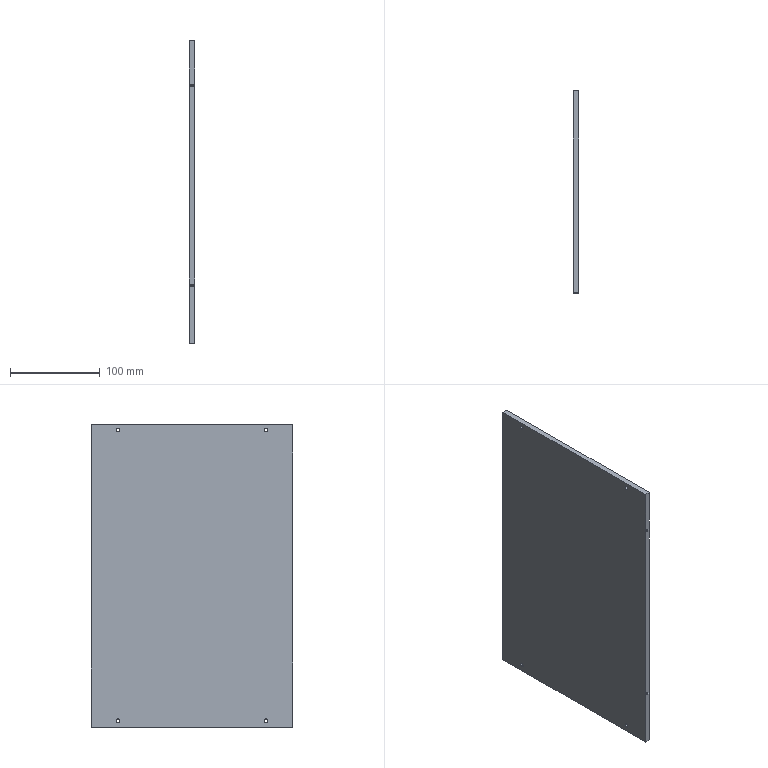Part | SolidWorks | features BaseBody 1 | 1 solid | 46 faces | box 6 x 225 x 337.5 mm | volume 454718 mm3 | cylinder 22 | cone 12 | plane 12 | commonest cylinder face diameters 4.2 x12 2.5 x6 4.11 x4